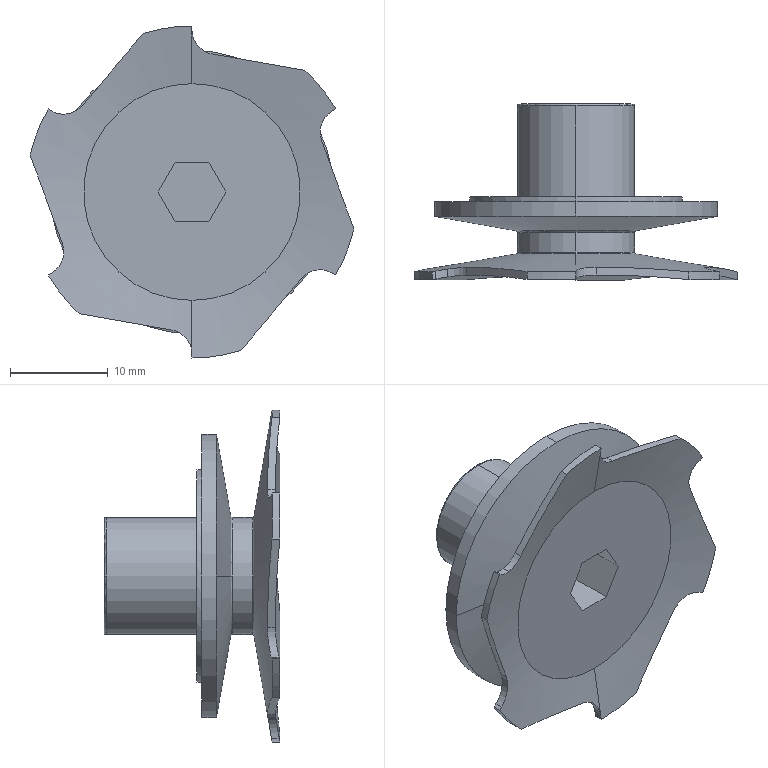Part | SolidWorks | features BaseBody 1 | 1 solid | 73 faces | box 33.147 x 18 x 34 mm | volume 3162 mm3 | cylinder 25 | plane 24 | torus 14 | cone 10 | commonest cylinder face diameters 5 x7 34 x6 12 x4 6.647 x2 18.5 x2 21.8 x2